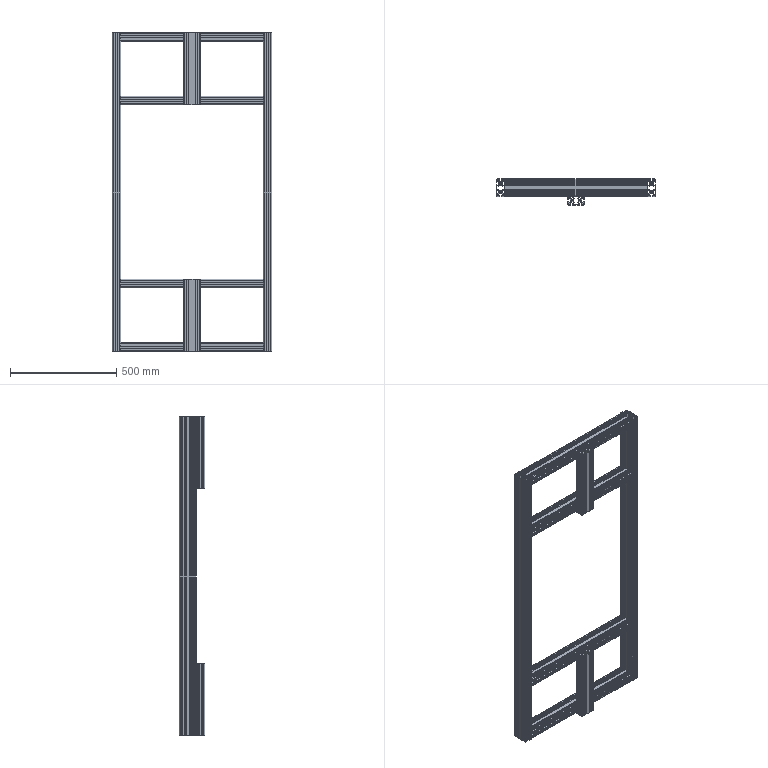Part | SolidWorks | 8 solids | 1240 faces | box 750.002 x 120.002 x 1500 mm | volume 6260738 mm3 | plane 1136 | cylinder 104 | commonest cylinder face diameters 9 x40 5 x32 6.8 x32